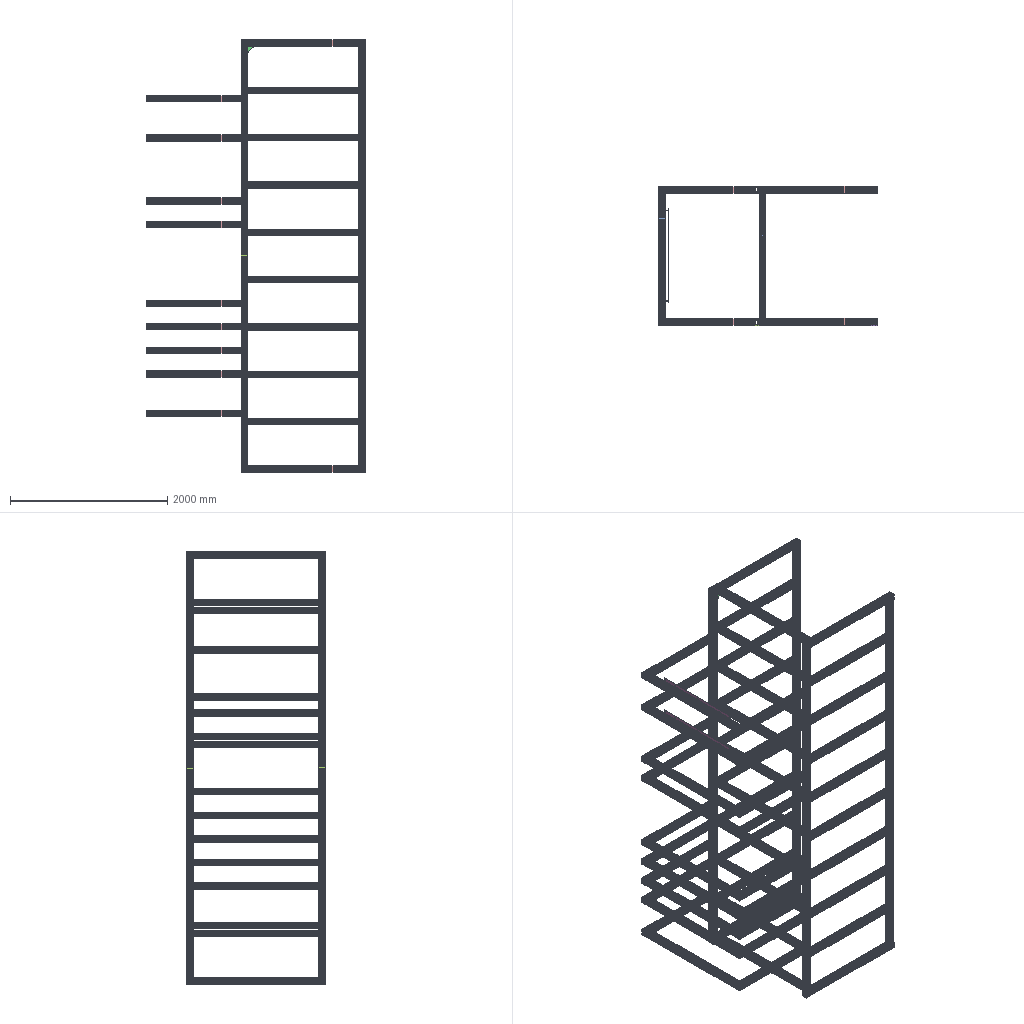Assembly | SolidWorks | 9 different items | 68 placed | box 2780 x 1760 x 5500 mm
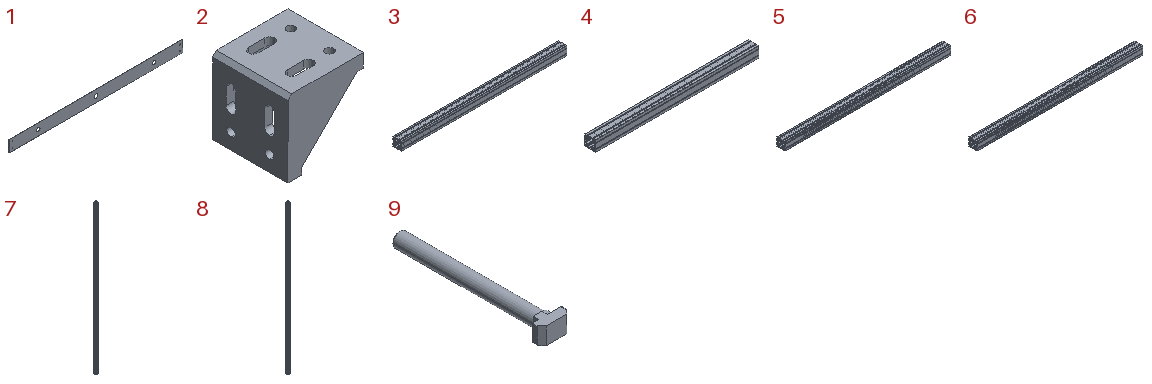Parts list (item | quantity | size | volume | features):
1 | x2 | 1200 x 2 x 80 mm | 188829 mm3 | features Extrusion 1
2 | x1 | 78 x 78 x 78 mm | 101387 mm3 | features ICE 11, HoleWzd 2, Chamfer 1, Extrusion 1
3 | x20 | 1500 x 80 x 80 mm | 3433531 mm3 | features ICE 1, WeldMemberFeat 1, WeldmentFeature 1
4 | x18 | 1200 x 80 x 80 mm | 2746825 mm3 | features ICE 1, WeldMemberFeat 1, WeldmentFeature 1
5 | x9 | 1600 x 80 x 80 mm | 3662433 mm3 | features ICE 1, WeldMemberFeat 1, WeldmentFeature 1
6 | x10 | 1600 x 80 x 80 mm | 3662433 mm3 | features ICE 1, WeldMemberFeat 1, WeldmentFeature 1
7 | x2 | 80 x 80 x 5338 mm | 9294002 mm3 | features Extrusion 1
8 | x2 | 80 x 80 x 5500 mm | 9576060 mm3 | features Extrusion 1
9 | x4 | 10.5 x 55.3 x 6 mm | 1236 mm3 | features Fillet 2, ICE 2, Chamfer 1, Extrusion 1, Revolution 1
Mates (type | each side: item.copy, entity, surface, feature):
Coincident | 3.1 face plane Aluminum profile 80 X 80G X R1.5(1) | 6.1 face plane Aluminum profile 80 X 80G X R1.5(1) | 3 times
Coincident | 3.1 face plane Aluminum profile 80 X 80G X R1.5(1) | 8.1 face plane Boss-Extrude1 | 3 times
Coincident | 3.2 face plane Aluminum profile 80 X 80G X R1.5(1) | 7.1 face plane Boss-Extrude1 | 3 times
Coincident | 3.2 face plane Aluminum profile 80 X 80G X R1.5(1) | 2.1 face plane Boss-Extrude2
Coincident | 8.2 face plane Boss-Extrude1 | 2.1 face plane Boss-Extrude4
Coincident | 3.2 face plane Aluminum profile 80 X 80G X R1.5(1) | 2.1 face plane Boss-Extrude1
Coincident | 8.2 face plane Boss-Extrude1 | 4.1 face plane Aluminum profile 80 X 80G X R1.5(1) | 2 times
DistanceDim | 4.1 face plane Aluminum profile 80 X 80G X R1.5(1) | 8.2 face plane Boss-Extrude1
Coincident | 8.2 face plane Boss-Extrude1 | 4.2 face plane Aluminum profile 80 X 80G X R1.5(1)
Coincident | 8.1 face plane Boss-Extrude1 | 4.2 face plane Aluminum profile 80 X 80G X R1.5(1)
DistanceDim | 4.2 face plane Aluminum profile 80 X 80G X R1.5(1) | 8.2 face plane Boss-Extrude1
Coincident | 4.2 face plane Aluminum profile 80 X 80G X R1.5(1) | 5.1 face plane Aluminum profile 80 X 80G X R1.5(1) | 3 times
Coincident | 5.1 face plane Aluminum profile 80 X 80G X R1.5(1) | 9.1 face plane Cut-Extrude1
Symmetric | 5.1 face plane Aluminum profile 80 X 80G X R1.5(1) | 5.1 face plane Aluminum profile 80 X 80G X R1.5(1) | 9.1 plane
DistanceDim | 5.1 face plane Aluminum profile 80 X 80G X R1.5(1) | 9.1 face plane Boss-Extrude1
Concentric | 9.1 face cylinder Revolve1 | 1.1 face cylinder Boss-Extrude1
Concentric | 9.2 face cylinder Revolve1 | 1.1 face cylinder Boss-Extrude1